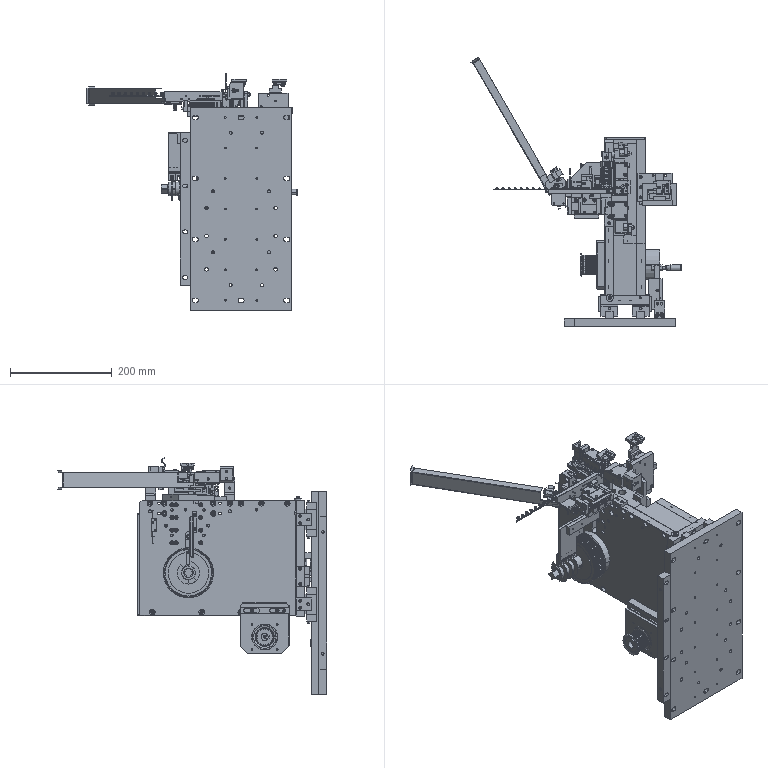Part | NX | 214 solids | 15349 faces | volume 6612443 mm3 | plane 8151 | cylinder 5142 | cone 1370 | torus 393 | spline 189 | sphere 104 | commonest cylinder face diameters 5 x551 0.3 x368 0.2 x334 0.5 x295 3.3 x284 2.5 x189